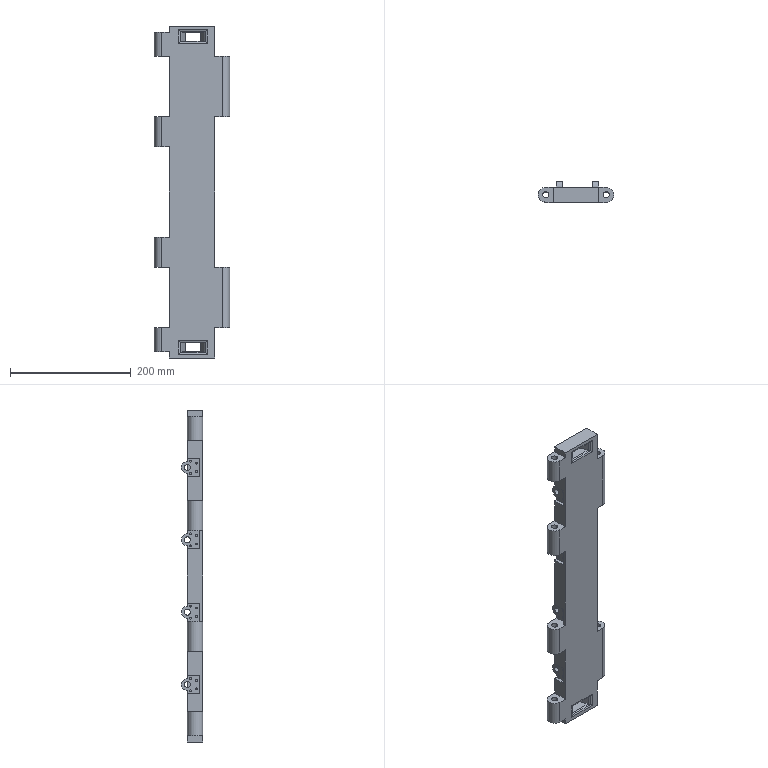Part | SolidWorks | features BaseBody 1 | 1 solid | 204 faces | box 125 x 35 x 550 mm | volume 741784 mm3 | cylinder 106 | plane 98 | commonest cylinder face diameters 3 x32 10 x28 8 x16 12 x16 20 x8 25 x6